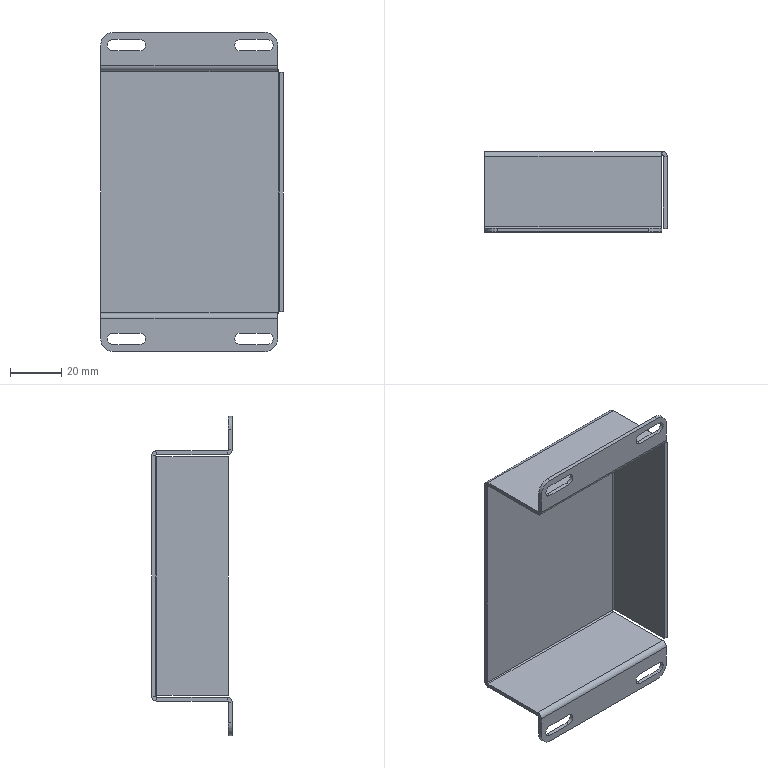Part | STEP file | 1 solid | 66 faces | box 71.5 x 31.5 x 125 mm | volume 22831 mm3 | plane 40 | cylinder 22 | spline 4 | commonest cylinder face diameters 4.5 x8 1 x5 4 x5 10 x4